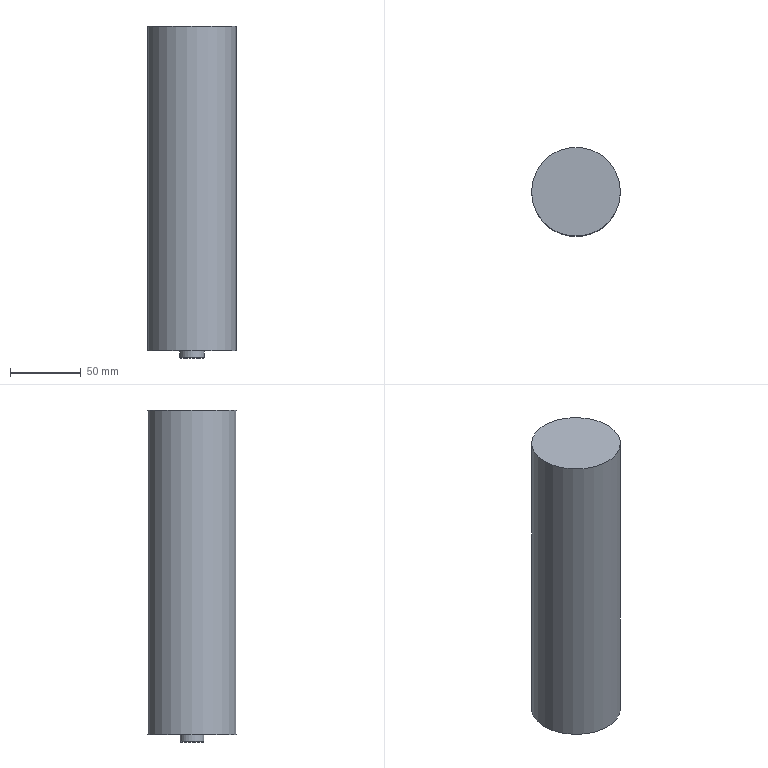Part | NX | features solid 2 | 1 solid | 6 faces | box 63 x 63 x 235 mm | volume 718095 mm3 | plane 3 | cylinder 2 | cone 1 | commonest cylinder face diameters 17 x1 63 x1
STEP:
#1=CARTESIAN_POINT('',(-1323.5,725.,250.));
#2=VERTEX_POINT('',#1);
#3=CARTESIAN_POINT('',(-1355.,725.,250.));
#4=DIRECTION('',(0.,0.,1.));
#5=DIRECTION('',(1.,0.,0.));
#6=AXIS2_PLACEMENT_3D('',#3,#4,#5);
#7=CIRCLE('',#6,31.5);
#8=EDGE_CURVE('',#2,#2,#7,.F.);
#9=ORIENTED_EDGE('',*,*,#8,.T.);
#10=EDGE_LOOP('',(#9));
#11=FACE_BOUND('',#10,.T.);
#12=CARTESIAN_POINT('',(-1323.5,725.,20.));
#13=VERTEX_POINT('',#12);
#14=CARTESIAN_POINT('',(-1355.,725.,20.));
#15=DIRECTION('',(0.,0.,-1.));
#16=DIRECTION('',(1.,0.,0.));
#17=AXIS2_PLACEMENT_3D('',#14,#15,#16);
#18=CIRCLE('',#17,31.5);
#19=EDGE_CURVE('',#13,#13,#18,.T.);
#20=ORIENTED_EDGE('',*,*,#19,.F.);
#21=EDGE_LOOP('',(#20));
#22=FACE_BOUND('',#21,.T.);
#23=CARTESIAN_POINT('',(-1355.,725.,200.));
#24=DIRECTION('',(0.,0.,-1.));
#25=DIRECTION('',(-1.,0.,0.));
#26=AXIS2_PLACEMENT_3D('',#23,#24,#25);
#27=CYLINDRICAL_SURFACE('',#26,31.5);
#28=ADVANCED_FACE('',(#11,#22),#27,.T.);
#29=ORIENTED_EDGE('',*,*,#8,.F.);
#30=EDGE_LOOP('',(#29));
#31=FACE_BOUND('',#30,.T.);
#32=CARTESIAN_POINT('',(-1355.,725.,250.));
#33=DIRECTION('',(0.,0.,1.));
#34=DIRECTION('',(1.,0.,0.));
#35=AXIS2_PLACEMENT_3D('',#32,#33,#34);
#36=PLANE('',#35);
#37=ADVANCED_FACE('',(#31),#36,.T.);
#38=CARTESIAN_POINT('',(-1363.5,725.,20.));
#39=VERTEX_POINT('',#38);
#40=CARTESIAN_POINT('',(-1355.,725.,20.));
#41=DIRECTION('',(0.,0.,1.));
#42=DIRECTION('',(-1.,0.,0.));
#43=AXIS2_PLACEMENT_3D('',#40,#41,#42);
#44=CIRCLE('',#43,8.5);
#45=EDGE_CURVE('',#39,#39,#44,.T.);
#46=ORIENTED_EDGE('',*,*,#45,.T.);
#47=EDGE_LOOP('',(#46));
#48=FACE_BOUND('',#47,.T.);
#49=ORIENTED_EDGE('',*,*,#19,.T.);
#50=EDGE_LOOP('',(#49));
#51=FACE_BOUND('',#50,.T.);
#52=CARTESIAN_POINT('',(-1355.,725.,20.));
#53=DIRECTION('',(0.,0.,1.));
#54=DIRECTION('',(1.,0.,0.));
#55=AXIS2_PLACEMENT_3D('',#52,#53,#54);
#56=PLANE('',#55);
#57=ADVANCED_FACE('',(#48,#51),#56,.F.);
#58=CARTESIAN_POINT('',(-1363.,725.,15.));
#59=VERTEX_POINT('',#58);
#60=CARTESIAN_POINT('',(-1355.,725.,15.));
#61=DIRECTION('',(0.,0.,1.));
#62=DIRECTION('',(-1.,0.,0.));
#63=AXIS2_PLACEMENT_3D('',#60,#61,#62);
#64=CIRCLE('',#63,8.);
#65=EDGE_CURVE('',#59,#59,#64,.T.);
#66=ORIENTED_EDGE('',*,*,#65,.F.);
#67=EDGE_LOOP('',(#66));
#68=FACE_BOUND('',#67,.T.);
#69=CARTESIAN_POINT('',(-1355.,725.,15.));
#70=DIRECTION('',(0.,0.,-1.));
#71=DIRECTION('',(-1.,0.,0.));
#72=AXIS2_PLACEMENT_3D('',#69,#70,#71);
#73=PLANE('',#72);
#74=ADVANCED_FACE('',(#68),#73,.T.);
#75=CARTESIAN_POINT('',(-1363.5,725.,15.5));
#76=VERTEX_POINT('',#75);
#77=CARTESIAN_POINT('',(-1355.,725.,15.5));
#78=DIRECTION('',(0.,0.,1.));
#79=DIRECTION('',(-1.,0.,0.));
#80=AXIS2_PLACEMENT_3D('',#77,#78,#79);
#81=CIRCLE('',#80,8.5);
#82=EDGE_CURVE('',#76,#76,#81,.F.);
#83=ORIENTED_EDGE('',*,*,#82,.F.);
#84=EDGE_LOOP('',(#83));
#85=FACE_BOUND('',#84,.T.);
#86=ORIENTED_EDGE('',*,*,#45,.F.);
#87=EDGE_LOOP('',(#86));
#88=FACE_BOUND('',#87,.T.);
#89=CARTESIAN_POINT('',(-1355.,725.,20.));
#90=DIRECTION('',(0.,0.,-1.));
#91=DIRECTION('',(-1.,0.,0.));
#92=AXIS2_PLACEMENT_3D('',#89,#90,#91);
#93=CYLINDRICAL_SURFACE('',#92,8.5);
#94=ADVANCED_FACE('',(#85,#88),#93,.T.);
#95=ORIENTED_EDGE('',*,*,#82,.T.);
#96=EDGE_LOOP('',(#95));
#97=FACE_BOUND('',#96,.T.);
#98=ORIENTED_EDGE('',*,*,#65,.T.);
#99=EDGE_LOOP('',(#98));
#100=FACE_BOUND('',#99,.T.);
#101=CARTESIAN_POINT('',(-1355.,725.,15.));
#102=DIRECTION('',(0.,0.,1.));
#103=DIRECTION('',(1.,0.,0.));
#104=AXIS2_PLACEMENT_3D('',#101,#102,#103);
#105=CONICAL_SURFACE('',#104,8.,0.7854);
#106=ADVANCED_FACE('',(#97,#100),#105,.T.);
#107=CLOSED_SHELL('',(#28,#37,#57,#74,#94,#106));
#108=MANIFOLD_SOLID_BREP('',#107);
#109=(LENGTH_UNIT()NAMED_UNIT(*)SI_UNIT(.MILLI.,.METRE.));
#110=UNCERTAINTY_MEASURE_WITH_UNIT(LENGTH_MEASURE(0.00001),#109,'','');
#111=(NAMED_UNIT(*)PLANE_ANGLE_UNIT()SI_UNIT($,.RADIAN.));
#112=(NAMED_UNIT(*)SI_UNIT($,.STERADIAN.)SOLID_ANGLE_UNIT());
#113=(GEOMETRIC_REPRESENTATION_CONTEXT(3)GLOBAL_UNCERTAINTY_ASSIGNED_CONTEXT((#110))GLOBAL_UNIT_ASSIGNED_CONTEXT((#109,#111,#112))REPRESENTATION_CONTEXT('',''));
#114=ADVANCED_BREP_SHAPE_REPRESENTATION('',(#108),#113);